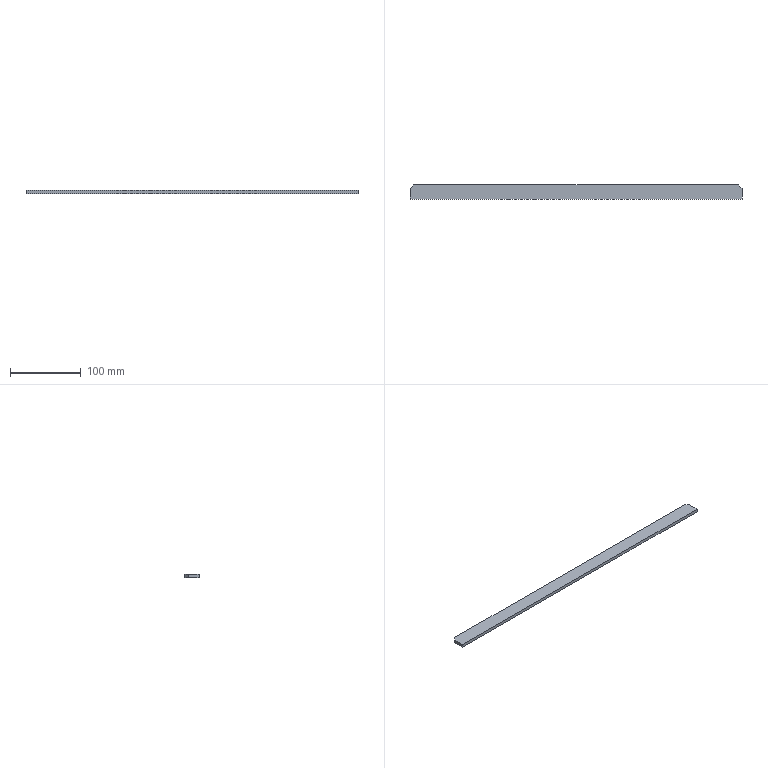Part | SolidWorks | features Chamfer 1, FlatPattern 1, SMBaseFlange 1, SheetMetal 1 | 1 solid | 8 faces | box 470 x 20 x 4.5 mm | volume 42188 mm3 | plane 8
STEP:
#1=CARTESIAN_POINT('',(235.,-10.,0.));
#2=VERTEX_POINT('',#1);
#3=CARTESIAN_POINT('',(235.,5.,0.));
#4=VERTEX_POINT('',#3);
#5=CARTESIAN_POINT('',(235.,10.,0.));
#6=DIRECTION('',(0.,1.,0.));
#7=VECTOR('',#6,1000.);
#8=LINE('',#5,#7);
#9=EDGE_CURVE('',#2,#4,#8,.T.);
#10=ORIENTED_EDGE('',*,*,#9,.T.);
#11=CARTESIAN_POINT('',(235.,5.,4.5));
#12=VERTEX_POINT('',#11);
#13=CARTESIAN_POINT('',(235.,5.,4.5));
#14=DIRECTION('',(0.,0.,1.));
#15=VECTOR('',#14,1000.);
#16=LINE('',#13,#15);
#17=EDGE_CURVE('',#4,#12,#16,.T.);
#18=ORIENTED_EDGE('',*,*,#17,.T.);
#19=CARTESIAN_POINT('',(235.,-10.,4.5));
#20=VERTEX_POINT('',#19);
#21=CARTESIAN_POINT('',(235.,10.,4.5));
#22=DIRECTION('',(0.,1.,0.));
#23=VECTOR('',#22,1000.);
#24=LINE('',#21,#23);
#25=EDGE_CURVE('',#20,#12,#24,.T.);
#26=ORIENTED_EDGE('',*,*,#25,.F.);
#27=CARTESIAN_POINT('',(235.,-10.,4.5));
#28=DIRECTION('',(0.,0.,-1.));
#29=VECTOR('',#28,1000.);
#30=LINE('',#27,#29);
#31=EDGE_CURVE('',#20,#2,#30,.T.);
#32=ORIENTED_EDGE('',*,*,#31,.T.);
#33=EDGE_LOOP('',(#10,#18,#26,#32));
#34=FACE_OUTER_BOUND('',#33,.T.);
#35=CARTESIAN_POINT('',(235.,10.,4.5));
#36=DIRECTION('',(-1.,0.,0.));
#37=DIRECTION('',(0.,0.,1.));
#38=AXIS2_PLACEMENT_3D('',#35,#36,#37);
#39=PLANE('',#38);
#40=ADVANCED_FACE('',(#34),#39,.F.);
#41=CARTESIAN_POINT('',(230.,10.,4.5));
#42=VERTEX_POINT('',#41);
#43=CARTESIAN_POINT('',(-230.,10.,4.5));
#44=VERTEX_POINT('',#43);
#45=CARTESIAN_POINT('',(-235.,10.,4.5));
#46=DIRECTION('',(-1.,0.,0.));
#47=VECTOR('',#46,1000.);
#48=LINE('',#45,#47);
#49=EDGE_CURVE('',#42,#44,#48,.T.);
#50=ORIENTED_EDGE('',*,*,#49,.F.);
#51=CARTESIAN_POINT('',(230.,10.,0.));
#52=VERTEX_POINT('',#51);
#53=CARTESIAN_POINT('',(230.,10.,4.5));
#54=DIRECTION('',(0.,0.,-1.));
#55=VECTOR('',#54,1000.);
#56=LINE('',#53,#55);
#57=EDGE_CURVE('',#42,#52,#56,.T.);
#58=ORIENTED_EDGE('',*,*,#57,.T.);
#59=CARTESIAN_POINT('',(-230.,10.,0.));
#60=VERTEX_POINT('',#59);
#61=CARTESIAN_POINT('',(-235.,10.,0.));
#62=DIRECTION('',(-1.,0.,0.));
#63=VECTOR('',#62,1000.);
#64=LINE('',#61,#63);
#65=EDGE_CURVE('',#52,#60,#64,.T.);
#66=ORIENTED_EDGE('',*,*,#65,.T.);
#67=CARTESIAN_POINT('',(-230.,10.,4.5));
#68=DIRECTION('',(0.,0.,1.));
#69=VECTOR('',#68,1000.);
#70=LINE('',#67,#69);
#71=EDGE_CURVE('',#60,#44,#70,.T.);
#72=ORIENTED_EDGE('',*,*,#71,.T.);
#73=EDGE_LOOP('',(#50,#58,#66,#72));
#74=FACE_OUTER_BOUND('',#73,.T.);
#75=CARTESIAN_POINT('',(-235.,10.,4.5));
#76=DIRECTION('',(0.,-1.,0.));
#77=DIRECTION('',(0.,0.,-1.));
#78=AXIS2_PLACEMENT_3D('',#75,#76,#77);
#79=PLANE('',#78);
#80=ADVANCED_FACE('',(#74),#79,.F.);
#81=CARTESIAN_POINT('',(-235.,5.,4.5));
#82=VERTEX_POINT('',#81);
#83=CARTESIAN_POINT('',(-235.,-10.,4.5));
#84=VERTEX_POINT('',#83);
#85=CARTESIAN_POINT('',(-235.,10.,4.5));
#86=DIRECTION('',(0.,-1.,0.));
#87=VECTOR('',#86,1000.);
#88=LINE('',#85,#87);
#89=EDGE_CURVE('',#82,#84,#88,.T.);
#90=ORIENTED_EDGE('',*,*,#89,.F.);
#91=CARTESIAN_POINT('',(-235.,5.,0.));
#92=VERTEX_POINT('',#91);
#93=CARTESIAN_POINT('',(-235.,5.,4.5));
#94=DIRECTION('',(0.,0.,-1.));
#95=VECTOR('',#94,1000.);
#96=LINE('',#93,#95);
#97=EDGE_CURVE('',#82,#92,#96,.T.);
#98=ORIENTED_EDGE('',*,*,#97,.T.);
#99=CARTESIAN_POINT('',(-235.,-10.,0.));
#100=VERTEX_POINT('',#99);
#101=CARTESIAN_POINT('',(-235.,10.,0.));
#102=DIRECTION('',(0.,-1.,0.));
#103=VECTOR('',#102,1000.);
#104=LINE('',#101,#103);
#105=EDGE_CURVE('',#92,#100,#104,.T.);
#106=ORIENTED_EDGE('',*,*,#105,.T.);
#107=CARTESIAN_POINT('',(-235.,-10.,4.5));
#108=DIRECTION('',(0.,0.,-1.));
#109=VECTOR('',#108,1000.);
#110=LINE('',#107,#109);
#111=EDGE_CURVE('',#84,#100,#110,.T.);
#112=ORIENTED_EDGE('',*,*,#111,.F.);
#113=EDGE_LOOP('',(#90,#98,#106,#112));
#114=FACE_OUTER_BOUND('',#113,.T.);
#115=CARTESIAN_POINT('',(-235.,10.,4.5));
#116=DIRECTION('',(1.,0.,0.));
#117=DIRECTION('',(0.,0.,-1.));
#118=AXIS2_PLACEMENT_3D('',#115,#116,#117);
#119=PLANE('',#118);
#120=ADVANCED_FACE('',(#114),#119,.F.);
#121=CARTESIAN_POINT('',(-235.,-10.,0.));
#122=DIRECTION('',(1.,0.,0.));
#123=VECTOR('',#122,1000.);
#124=LINE('',#121,#123);
#125=EDGE_CURVE('',#100,#2,#124,.T.);
#126=ORIENTED_EDGE('',*,*,#125,.T.);
#127=ORIENTED_EDGE('',*,*,#31,.F.);
#128=CARTESIAN_POINT('',(-235.,-10.,4.5));
#129=DIRECTION('',(1.,0.,0.));
#130=VECTOR('',#129,1000.);
#131=LINE('',#128,#130);
#132=EDGE_CURVE('',#84,#20,#131,.T.);
#133=ORIENTED_EDGE('',*,*,#132,.F.);
#134=ORIENTED_EDGE('',*,*,#111,.T.);
#135=EDGE_LOOP('',(#126,#127,#133,#134));
#136=FACE_OUTER_BOUND('',#135,.T.);
#137=CARTESIAN_POINT('',(-235.,-10.,4.5));
#138=DIRECTION('',(0.,1.,0.));
#139=DIRECTION('',(0.,0.,1.));
#140=AXIS2_PLACEMENT_3D('',#137,#138,#139);
#141=PLANE('',#140);
#142=ADVANCED_FACE('',(#136),#141,.F.);
#143=ORIENTED_EDGE('',*,*,#25,.T.);
#144=CARTESIAN_POINT('',(120.,120.,4.5));
#145=DIRECTION('',(-0.7071,0.7071,0.));
#146=VECTOR('',#145,1000.);
#147=LINE('',#144,#146);
#148=EDGE_CURVE('',#12,#42,#147,.T.);
#149=ORIENTED_EDGE('',*,*,#148,.T.);
#150=ORIENTED_EDGE('',*,*,#49,.T.);
#151=CARTESIAN_POINT('',(-120.,120.,4.5));
#152=DIRECTION('',(-0.7071,-0.7071,0.));
#153=VECTOR('',#152,1000.);
#154=LINE('',#151,#153);
#155=EDGE_CURVE('',#44,#82,#154,.T.);
#156=ORIENTED_EDGE('',*,*,#155,.T.);
#157=ORIENTED_EDGE('',*,*,#89,.T.);
#158=ORIENTED_EDGE('',*,*,#132,.T.);
#159=EDGE_LOOP('',(#143,#149,#150,#156,#157,#158));
#160=FACE_OUTER_BOUND('',#159,.T.);
#161=CARTESIAN_POINT('',(0.,0.,4.5));
#162=DIRECTION('',(0.,0.,1.));
#163=DIRECTION('',(1.,0.,0.));
#164=AXIS2_PLACEMENT_3D('',#161,#162,#163);
#165=PLANE('',#164);
#166=ADVANCED_FACE('',(#160),#165,.T.);
#167=ORIENTED_EDGE('',*,*,#65,.F.);
#168=CARTESIAN_POINT('',(230.,10.,0.));
#169=DIRECTION('',(0.7071,-0.7071,0.));
#170=VECTOR('',#169,1000.);
#171=LINE('',#168,#170);
#172=EDGE_CURVE('',#52,#4,#171,.T.);
#173=ORIENTED_EDGE('',*,*,#172,.T.);
#174=ORIENTED_EDGE('',*,*,#9,.F.);
#175=ORIENTED_EDGE('',*,*,#125,.F.);
#176=ORIENTED_EDGE('',*,*,#105,.F.);
#177=CARTESIAN_POINT('',(-235.,5.,0.));
#178=DIRECTION('',(0.7071,0.7071,0.));
#179=VECTOR('',#178,1000.);
#180=LINE('',#177,#179);
#181=EDGE_CURVE('',#92,#60,#180,.T.);
#182=ORIENTED_EDGE('',*,*,#181,.T.);
#183=EDGE_LOOP('',(#167,#173,#174,#175,#176,#182));
#184=FACE_OUTER_BOUND('',#183,.T.);
#185=CARTESIAN_POINT('',(0.,0.,0.));
#186=DIRECTION('',(0.,0.,1.));
#187=DIRECTION('',(1.,0.,0.));
#188=AXIS2_PLACEMENT_3D('',#185,#186,#187);
#189=PLANE('',#188);
#190=ADVANCED_FACE('',(#184),#189,.F.);
#191=ORIENTED_EDGE('',*,*,#148,.F.);
#192=ORIENTED_EDGE('',*,*,#17,.F.);
#193=ORIENTED_EDGE('',*,*,#172,.F.);
#194=ORIENTED_EDGE('',*,*,#57,.F.);
#195=EDGE_LOOP('',(#191,#192,#193,#194));
#196=FACE_OUTER_BOUND('',#195,.T.);
#197=CARTESIAN_POINT('',(230.,10.,4.5));
#198=DIRECTION('',(-0.7071,-0.7071,0.));
#199=DIRECTION('',(0.,0.,-1.));
#200=AXIS2_PLACEMENT_3D('',#197,#198,#199);
#201=PLANE('',#200);
#202=ADVANCED_FACE('',(#196),#201,.F.);
#203=ORIENTED_EDGE('',*,*,#155,.F.);
#204=ORIENTED_EDGE('',*,*,#71,.F.);
#205=ORIENTED_EDGE('',*,*,#181,.F.);
#206=ORIENTED_EDGE('',*,*,#97,.F.);
#207=EDGE_LOOP('',(#203,#204,#205,#206));
#208=FACE_OUTER_BOUND('',#207,.T.);
#209=CARTESIAN_POINT('',(-235.,5.,4.5));
#210=DIRECTION('',(0.7071,-0.7071,0.));
#211=DIRECTION('',(0.,0.,-1.));
#212=AXIS2_PLACEMENT_3D('',#209,#210,#211);
#213=PLANE('',#212);
#214=ADVANCED_FACE('',(#208),#213,.F.);
#215=CLOSED_SHELL('',(#40,#80,#120,#142,#166,#190,#202,#214));
#216=MANIFOLD_SOLID_BREP('',#215);
#217=CARTESIAN_POINT('',(0.,0.,0.));
#218=DIRECTION('',(0.,0.,1.));
#219=DIRECTION('',(1.,0.,0.));
#220=AXIS2_PLACEMENT_3D('',#217,#218,#219);
#221=(LENGTH_UNIT()NAMED_UNIT(*)SI_UNIT(.MILLI.,.METRE.));
#222=UNCERTAINTY_MEASURE_WITH_UNIT(LENGTH_MEASURE(0.00001),#221,'','');
#223=(NAMED_UNIT(*)PLANE_ANGLE_UNIT()SI_UNIT($,.RADIAN.));
#224=(NAMED_UNIT(*)SI_UNIT($,.STERADIAN.)SOLID_ANGLE_UNIT());
#225=(GEOMETRIC_REPRESENTATION_CONTEXT(3)GLOBAL_UNCERTAINTY_ASSIGNED_CONTEXT((#222))GLOBAL_UNIT_ASSIGNED_CONTEXT((#221,#223,#224))REPRESENTATION_CONTEXT('',''));
#226=ADVANCED_BREP_SHAPE_REPRESENTATION('',(#216,#220),#225);